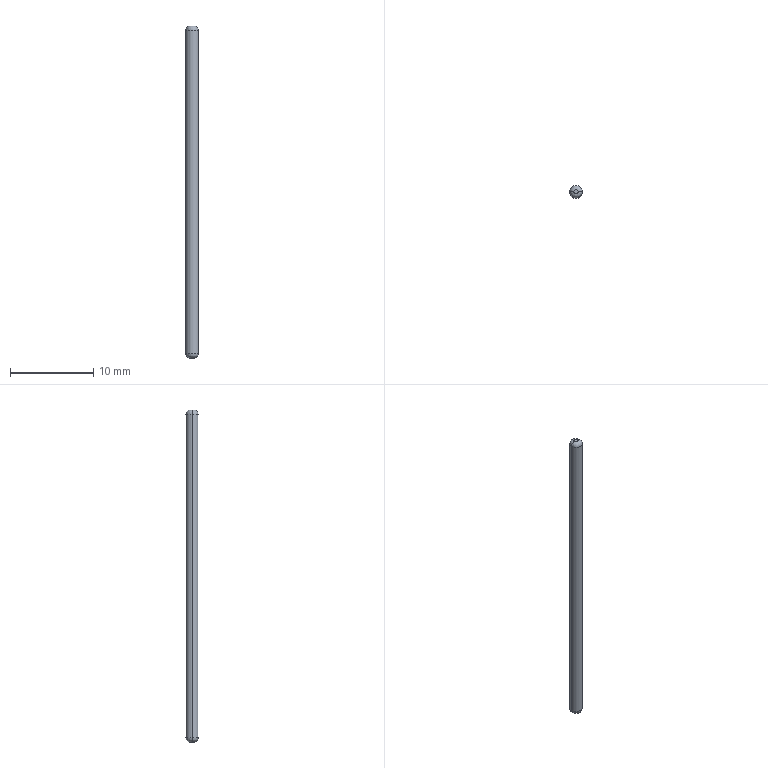Part | SolidWorks | features Extrusion 1, Fillet 1 | 1 solid | 8 faces | box 1.5 x 1.5 x 40 mm | volume 70.255 mm3 | torus 4 | cylinder 2 | plane 2 | commonest cylinder face diameters 1.5 x2
STEP:
#1=CARTESIAN_POINT('',(-0.75,0.,39.5));
#2=VERTEX_POINT('',#1);
#3=CARTESIAN_POINT('',(0.75,0.,39.5));
#4=VERTEX_POINT('',#3);
#5=CARTESIAN_POINT('',(0.,0.,39.5));
#6=DIRECTION('',(0.,0.,-1.));
#7=DIRECTION('',(1.,0.,0.));
#8=AXIS2_PLACEMENT_3D('',#5,#6,#7);
#9=CIRCLE('',#8,0.75);
#10=EDGE_CURVE('',#2,#4,#9,.T.);
#11=ORIENTED_EDGE('',*,*,#10,.F.);
#12=CARTESIAN_POINT('',(-0.25,0.,40.));
#13=VERTEX_POINT('',#12);
#14=CARTESIAN_POINT('',(-0.25,0.,39.5));
#15=DIRECTION('',(0.,1.,0.));
#16=DIRECTION('',(-1.,0.,0.));
#17=AXIS2_PLACEMENT_3D('',#14,#15,#16);
#18=CIRCLE('',#17,0.5);
#19=EDGE_CURVE('',#2,#13,#18,.T.);
#20=ORIENTED_EDGE('',*,*,#19,.T.);
#21=CARTESIAN_POINT('',(0.25,0.,40.));
#22=VERTEX_POINT('',#21);
#23=CARTESIAN_POINT('',(0.,0.,40.));
#24=DIRECTION('',(0.,0.,1.));
#25=DIRECTION('',(1.,0.,0.));
#26=AXIS2_PLACEMENT_3D('',#23,#24,#25);
#27=CIRCLE('',#26,0.25);
#28=EDGE_CURVE('',#22,#13,#27,.T.);
#29=ORIENTED_EDGE('',*,*,#28,.F.);
#30=CARTESIAN_POINT('',(0.25,0.,39.5));
#31=DIRECTION('',(0.,-1.,0.));
#32=DIRECTION('',(0.,0.,-1.));
#33=AXIS2_PLACEMENT_3D('',#30,#31,#32);
#34=CIRCLE('',#33,0.5);
#35=EDGE_CURVE('',#4,#22,#34,.T.);
#36=ORIENTED_EDGE('',*,*,#35,.F.);
#37=EDGE_LOOP('',(#11,#20,#29,#36));
#38=FACE_OUTER_BOUND('',#37,.T.);
#39=CARTESIAN_POINT('',(0.,0.,39.5));
#40=DIRECTION('',(0.,0.,1.));
#41=DIRECTION('',(1.,0.,0.));
#42=AXIS2_PLACEMENT_3D('',#39,#40,#41);
#43=TOROIDAL_SURFACE('',#42,0.25,0.5);
#44=ADVANCED_FACE('',(#38),#43,.T.);
#45=CARTESIAN_POINT('',(-0.25,0.,0.));
#46=VERTEX_POINT('',#45);
#47=CARTESIAN_POINT('',(0.25,0.,0.));
#48=VERTEX_POINT('',#47);
#49=CARTESIAN_POINT('',(0.,0.,0.));
#50=DIRECTION('',(0.,0.,-1.));
#51=DIRECTION('',(1.,0.,0.));
#52=AXIS2_PLACEMENT_3D('',#49,#50,#51);
#53=CIRCLE('',#52,0.25);
#54=EDGE_CURVE('',#46,#48,#53,.T.);
#55=ORIENTED_EDGE('',*,*,#54,.F.);
#56=CARTESIAN_POINT('',(-0.75,0.,0.5));
#57=VERTEX_POINT('',#56);
#58=CARTESIAN_POINT('',(-0.25,0.,0.5));
#59=DIRECTION('',(0.,1.,0.));
#60=DIRECTION('',(-1.,0.,0.));
#61=AXIS2_PLACEMENT_3D('',#58,#59,#60);
#62=CIRCLE('',#61,0.5);
#63=EDGE_CURVE('',#46,#57,#62,.T.);
#64=ORIENTED_EDGE('',*,*,#63,.T.);
#65=CARTESIAN_POINT('',(0.75,0.,0.5));
#66=VERTEX_POINT('',#65);
#67=CARTESIAN_POINT('',(0.,0.,0.5));
#68=DIRECTION('',(0.,0.,1.));
#69=DIRECTION('',(1.,0.,0.));
#70=AXIS2_PLACEMENT_3D('',#67,#68,#69);
#71=CIRCLE('',#70,0.75);
#72=EDGE_CURVE('',#66,#57,#71,.T.);
#73=ORIENTED_EDGE('',*,*,#72,.F.);
#74=CARTESIAN_POINT('',(0.25,0.,0.5));
#75=DIRECTION('',(0.,-1.,0.));
#76=DIRECTION('',(0.,0.,-1.));
#77=AXIS2_PLACEMENT_3D('',#74,#75,#76);
#78=CIRCLE('',#77,0.5);
#79=EDGE_CURVE('',#48,#66,#78,.T.);
#80=ORIENTED_EDGE('',*,*,#79,.F.);
#81=EDGE_LOOP('',(#55,#64,#73,#80));
#82=FACE_OUTER_BOUND('',#81,.T.);
#83=CARTESIAN_POINT('',(0.,0.,0.5));
#84=DIRECTION('',(0.,0.,1.));
#85=DIRECTION('',(1.,0.,0.));
#86=AXIS2_PLACEMENT_3D('',#83,#84,#85);
#87=TOROIDAL_SURFACE('',#86,0.25,0.5);
#88=ADVANCED_FACE('',(#82),#87,.T.);
#89=ORIENTED_EDGE('',*,*,#10,.T.);
#90=CARTESIAN_POINT('',(0.75,0.,40.));
#91=DIRECTION('',(0.,0.,-1.));
#92=VECTOR('',#91,1000.);
#93=LINE('',#90,#92);
#94=EDGE_CURVE('',#4,#66,#93,.T.);
#95=ORIENTED_EDGE('',*,*,#94,.T.);
#96=ORIENTED_EDGE('',*,*,#72,.T.);
#97=CARTESIAN_POINT('',(-0.75,0.,40.));
#98=DIRECTION('',(0.,0.,-1.));
#99=VECTOR('',#98,1000.);
#100=LINE('',#97,#99);
#101=EDGE_CURVE('',#2,#57,#100,.T.);
#102=ORIENTED_EDGE('',*,*,#101,.F.);
#103=EDGE_LOOP('',(#89,#95,#96,#102));
#104=FACE_OUTER_BOUND('',#103,.T.);
#105=CARTESIAN_POINT('',(0.,0.,40.));
#106=DIRECTION('',(0.,0.,-1.));
#107=DIRECTION('',(-1.,0.,0.));
#108=AXIS2_PLACEMENT_3D('',#105,#106,#107);
#109=CYLINDRICAL_SURFACE('',#108,0.75);
#110=ADVANCED_FACE('',(#104),#109,.T.);
#111=ORIENTED_EDGE('',*,*,#94,.F.);
#112=CARTESIAN_POINT('',(0.,0.,39.5));
#113=DIRECTION('',(0.,0.,-1.));
#114=DIRECTION('',(1.,0.,0.));
#115=AXIS2_PLACEMENT_3D('',#112,#113,#114);
#116=CIRCLE('',#115,0.75);
#117=EDGE_CURVE('',#4,#2,#116,.T.);
#118=ORIENTED_EDGE('',*,*,#117,.T.);
#119=ORIENTED_EDGE('',*,*,#101,.T.);
#120=CARTESIAN_POINT('',(0.,0.,0.5));
#121=DIRECTION('',(0.,0.,1.));
#122=DIRECTION('',(1.,0.,0.));
#123=AXIS2_PLACEMENT_3D('',#120,#121,#122);
#124=CIRCLE('',#123,0.75);
#125=EDGE_CURVE('',#57,#66,#124,.T.);
#126=ORIENTED_EDGE('',*,*,#125,.T.);
#127=EDGE_LOOP('',(#111,#118,#119,#126));
#128=FACE_OUTER_BOUND('',#127,.T.);
#129=CARTESIAN_POINT('',(0.,0.,40.));
#130=DIRECTION('',(0.,0.,-1.));
#131=DIRECTION('',(-1.,0.,0.));
#132=AXIS2_PLACEMENT_3D('',#129,#130,#131);
#133=CYLINDRICAL_SURFACE('',#132,0.75);
#134=ADVANCED_FACE('',(#128),#133,.T.);
#135=ORIENTED_EDGE('',*,*,#28,.T.);
#136=CARTESIAN_POINT('',(0.,0.,40.));
#137=DIRECTION('',(0.,0.,1.));
#138=DIRECTION('',(1.,0.,0.));
#139=AXIS2_PLACEMENT_3D('',#136,#137,#138);
#140=CIRCLE('',#139,0.25);
#141=EDGE_CURVE('',#13,#22,#140,.T.);
#142=ORIENTED_EDGE('',*,*,#141,.T.);
#143=EDGE_LOOP('',(#135,#142));
#144=FACE_OUTER_BOUND('',#143,.T.);
#145=CARTESIAN_POINT('',(0.,0.,40.));
#146=DIRECTION('',(0.,0.,1.));
#147=DIRECTION('',(1.,0.,0.));
#148=AXIS2_PLACEMENT_3D('',#145,#146,#147);
#149=PLANE('',#148);
#150=ADVANCED_FACE('',(#144),#149,.T.);
#151=CARTESIAN_POINT('',(0.,0.,0.));
#152=DIRECTION('',(0.,0.,-1.));
#153=DIRECTION('',(1.,0.,0.));
#154=AXIS2_PLACEMENT_3D('',#151,#152,#153);
#155=CIRCLE('',#154,0.25);
#156=EDGE_CURVE('',#48,#46,#155,.T.);
#157=ORIENTED_EDGE('',*,*,#156,.T.);
#158=ORIENTED_EDGE('',*,*,#54,.T.);
#159=EDGE_LOOP('',(#157,#158));
#160=FACE_OUTER_BOUND('',#159,.T.);
#161=CARTESIAN_POINT('',(0.,0.,0.));
#162=DIRECTION('',(0.,0.,1.));
#163=DIRECTION('',(1.,0.,0.));
#164=AXIS2_PLACEMENT_3D('',#161,#162,#163);
#165=PLANE('',#164);
#166=ADVANCED_FACE('',(#160),#165,.F.);
#167=ORIENTED_EDGE('',*,*,#63,.F.);
#168=ORIENTED_EDGE('',*,*,#156,.F.);
#169=ORIENTED_EDGE('',*,*,#79,.T.);
#170=ORIENTED_EDGE('',*,*,#125,.F.);
#171=EDGE_LOOP('',(#167,#168,#169,#170));
#172=FACE_OUTER_BOUND('',#171,.T.);
#173=CARTESIAN_POINT('',(0.,0.,0.5));
#174=DIRECTION('',(0.,0.,1.));
#175=DIRECTION('',(1.,0.,0.));
#176=AXIS2_PLACEMENT_3D('',#173,#174,#175);
#177=TOROIDAL_SURFACE('',#176,0.25,0.5);
#178=ADVANCED_FACE('',(#172),#177,.T.);
#179=ORIENTED_EDGE('',*,*,#19,.F.);
#180=ORIENTED_EDGE('',*,*,#117,.F.);
#181=ORIENTED_EDGE('',*,*,#35,.T.);
#182=ORIENTED_EDGE('',*,*,#141,.F.);
#183=EDGE_LOOP('',(#179,#180,#181,#182));
#184=FACE_OUTER_BOUND('',#183,.T.);
#185=CARTESIAN_POINT('',(0.,0.,39.5));
#186=DIRECTION('',(0.,0.,1.));
#187=DIRECTION('',(1.,0.,0.));
#188=AXIS2_PLACEMENT_3D('',#185,#186,#187);
#189=TOROIDAL_SURFACE('',#188,0.25,0.5);
#190=ADVANCED_FACE('',(#184),#189,.T.);
#191=CLOSED_SHELL('',(#44,#88,#110,#134,#150,#166,#178,#190));
#192=MANIFOLD_SOLID_BREP('',#191);
#193=CARTESIAN_POINT('',(0.,0.,0.));
#194=DIRECTION('',(0.,0.,1.));
#195=DIRECTION('',(1.,0.,0.));
#196=AXIS2_PLACEMENT_3D('',#193,#194,#195);
#197=(LENGTH_UNIT()NAMED_UNIT(*)SI_UNIT(.MILLI.,.METRE.));
#198=UNCERTAINTY_MEASURE_WITH_UNIT(LENGTH_MEASURE(0.00001),#197,'','');
#199=(NAMED_UNIT(*)PLANE_ANGLE_UNIT()SI_UNIT($,.RADIAN.));
#200=(NAMED_UNIT(*)SI_UNIT($,.STERADIAN.)SOLID_ANGLE_UNIT());
#201=(GEOMETRIC_REPRESENTATION_CONTEXT(3)GLOBAL_UNCERTAINTY_ASSIGNED_CONTEXT((#198))GLOBAL_UNIT_ASSIGNED_CONTEXT((#197,#199,#200))REPRESENTATION_CONTEXT('',''));
#202=ADVANCED_BREP_SHAPE_REPRESENTATION('',(#192,#196),#201);